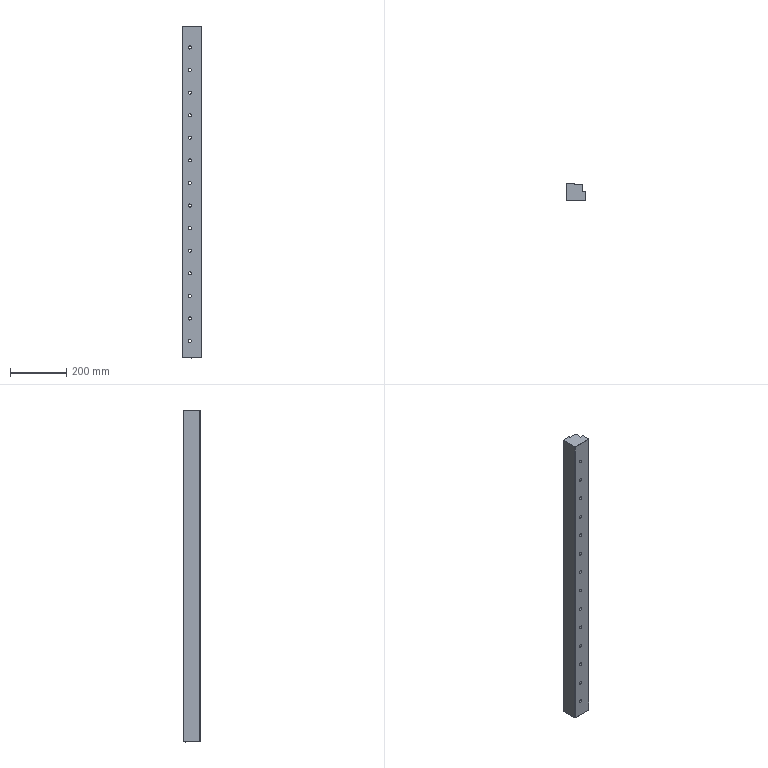Part | SolidWorks | features BaseBody 1 | 1 solid | 262 faces | box 70 x 60 x 1176 mm | volume 4173927 mm3 | cylinder 144 | plane 115 | cone 3 | commonest cylinder face diameters 6.5 x58 2 x30 11 x28 17.5 x28